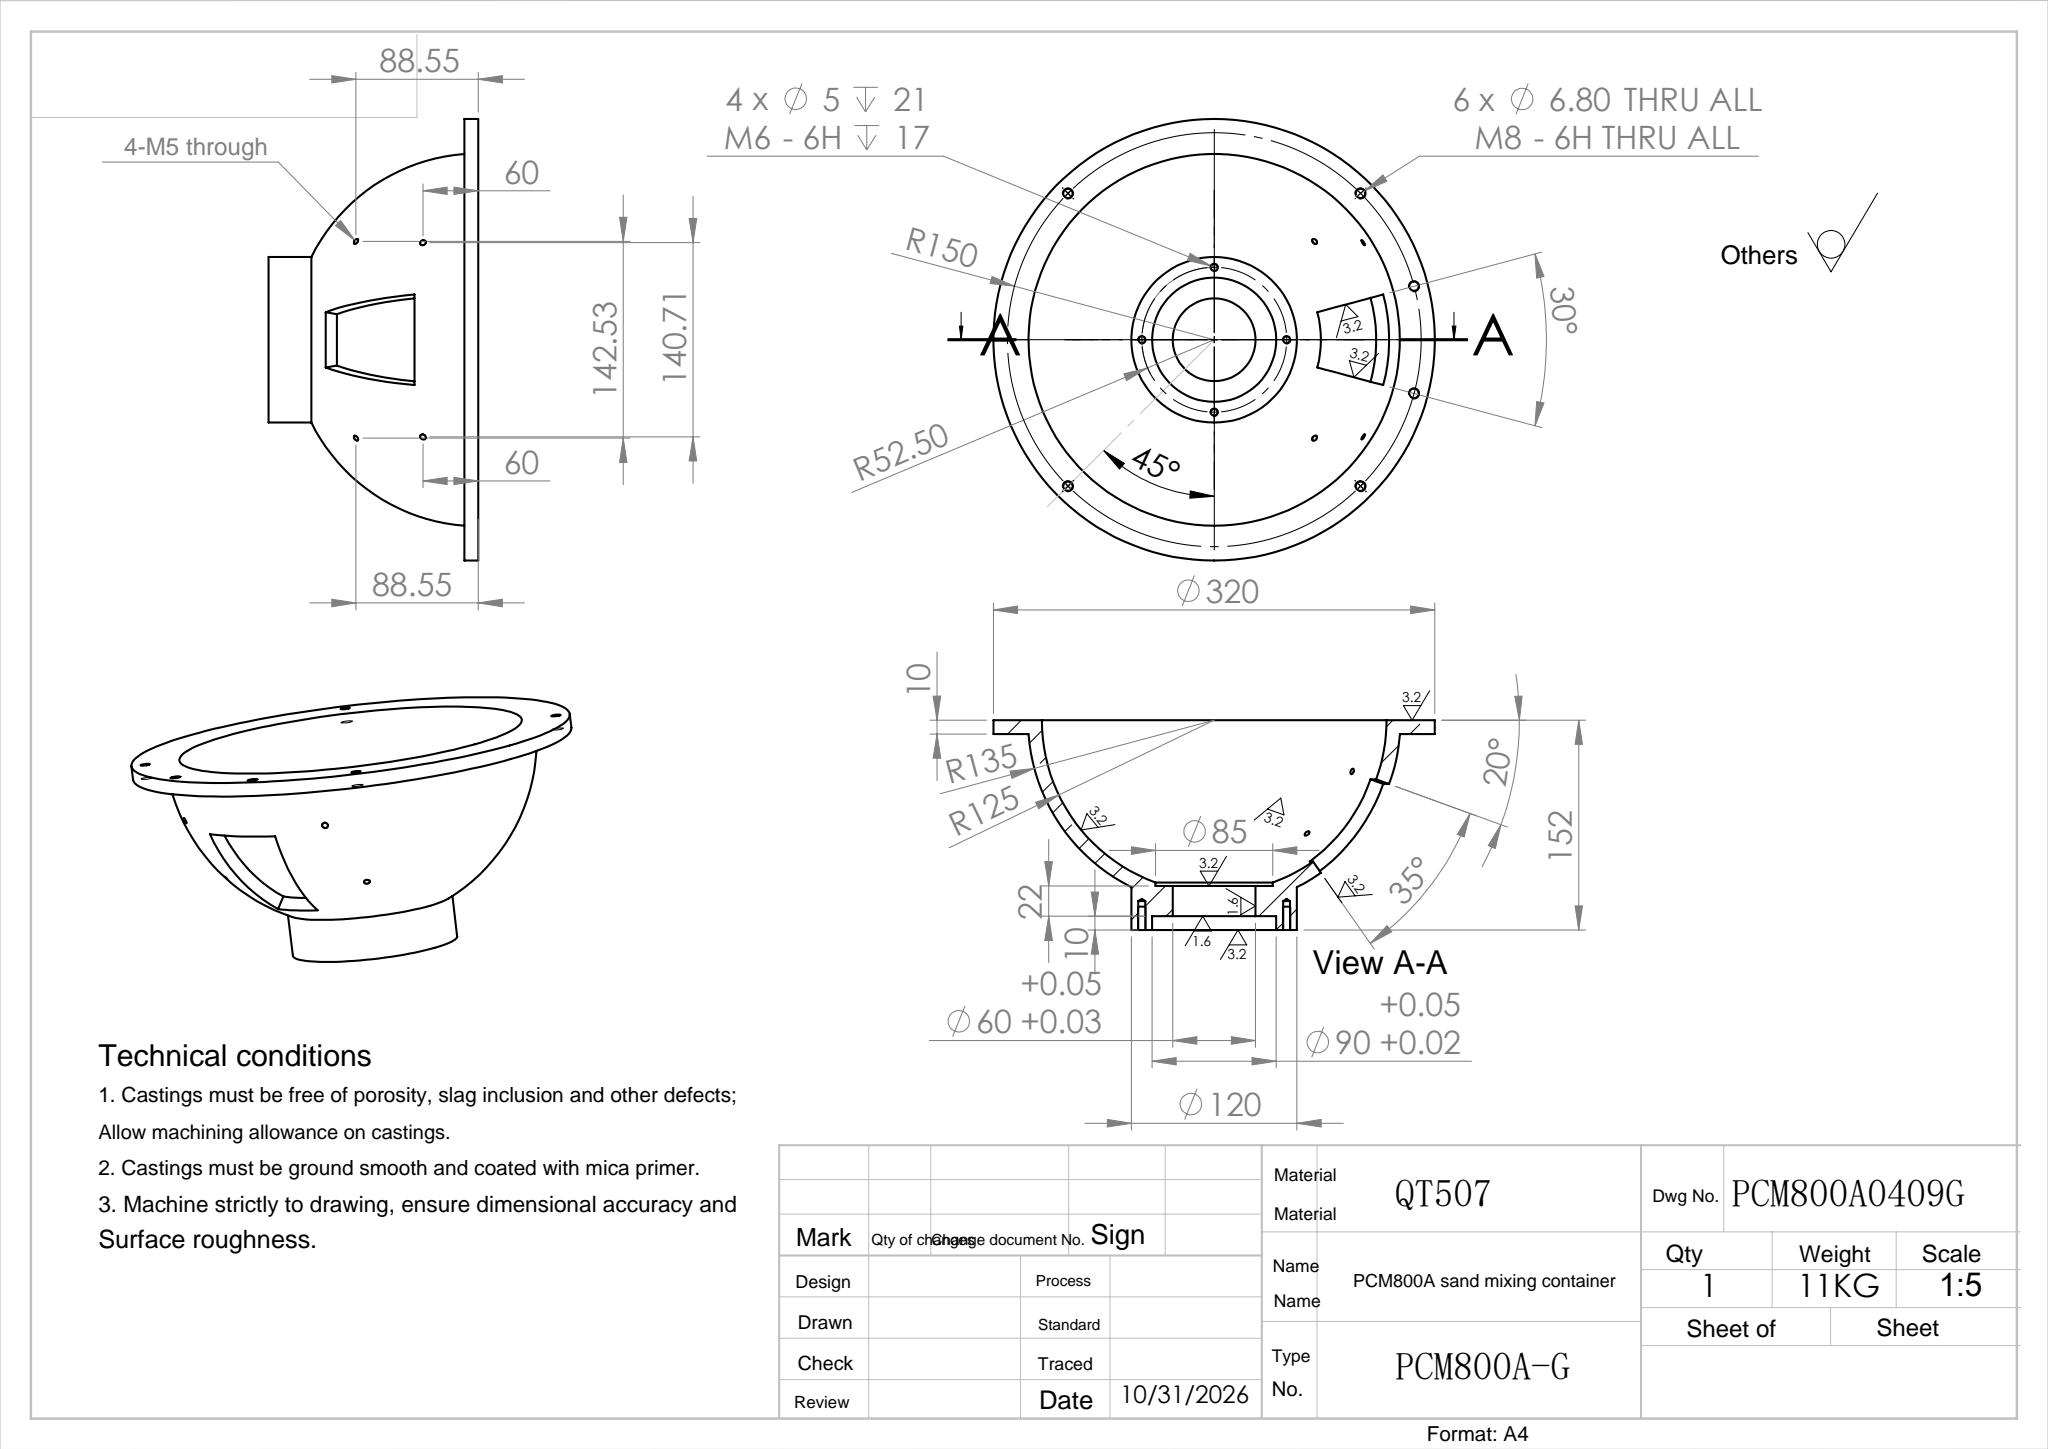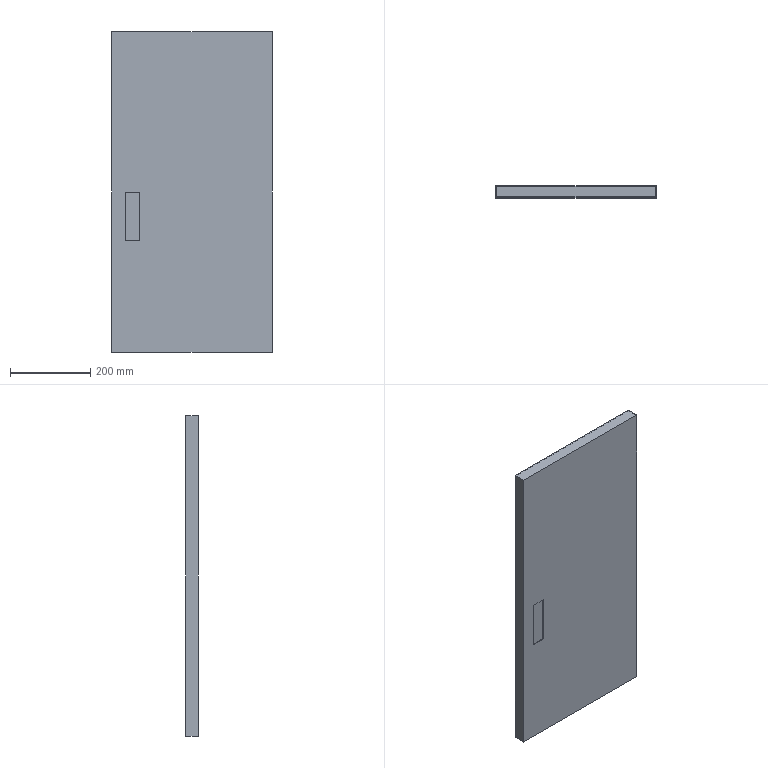Part | SolidWorks | features ICE 2, Extrusion 1, Shell 1 | 1 solid | 16 faces | box 400 x 30 x 800 mm | volume 1395984 mm3 | plane 16
STEP:
#1=CARTESIAN_POINT('',(2.,28.,-798.));
#2=VERTEX_POINT('',#1);
#3=CARTESIAN_POINT('',(2.,2.,-798.));
#4=VERTEX_POINT('',#3);
#5=CARTESIAN_POINT('',(2.,30.,-798.));
#6=DIRECTION('',(0.,-1.,0.));
#7=VECTOR('',#6,1000.);
#8=LINE('',#5,#7);
#9=EDGE_CURVE('',#2,#4,#8,.T.);
#10=ORIENTED_EDGE('',*,*,#9,.F.);
#11=CARTESIAN_POINT('',(2.,28.,-2.));
#12=VERTEX_POINT('',#11);
#13=CARTESIAN_POINT('',(2.,28.,0.));
#14=DIRECTION('',(0.,0.,1.));
#15=VECTOR('',#14,1000.);
#16=LINE('',#13,#15);
#17=EDGE_CURVE('',#2,#12,#16,.T.);
#18=ORIENTED_EDGE('',*,*,#17,.T.);
#19=CARTESIAN_POINT('',(2.,2.,-2.));
#20=VERTEX_POINT('',#19);
#21=CARTESIAN_POINT('',(2.,30.,-2.));
#22=DIRECTION('',(0.,-1.,0.));
#23=VECTOR('',#22,1000.);
#24=LINE('',#21,#23);
#25=EDGE_CURVE('',#12,#20,#24,.T.);
#26=ORIENTED_EDGE('',*,*,#25,.T.);
#27=CARTESIAN_POINT('',(2.,2.,-800.));
#28=DIRECTION('',(0.,0.,1.));
#29=VECTOR('',#28,1000.);
#30=LINE('',#27,#29);
#31=EDGE_CURVE('',#4,#20,#30,.T.);
#32=ORIENTED_EDGE('',*,*,#31,.F.);
#33=EDGE_LOOP('',(#10,#18,#26,#32));
#34=FACE_OUTER_BOUND('',#33,.T.);
#35=CARTESIAN_POINT('',(2.,30.,0.));
#36=DIRECTION('',(1.,0.,0.));
#37=DIRECTION('',(0.,0.,-1.));
#38=AXIS2_PLACEMENT_3D('',#35,#36,#37);
#39=PLANE('',#38);
#40=ADVANCED_FACE('',(#34),#39,.T.);
#41=ORIENTED_EDGE('',*,*,#25,.F.);
#42=CARTESIAN_POINT('',(398.,28.,-2.));
#43=VERTEX_POINT('',#42);
#44=CARTESIAN_POINT('',(0.,28.,-2.));
#45=DIRECTION('',(1.,0.,0.));
#46=VECTOR('',#45,1000.);
#47=LINE('',#44,#46);
#48=EDGE_CURVE('',#12,#43,#47,.T.);
#49=ORIENTED_EDGE('',*,*,#48,.T.);
#50=CARTESIAN_POINT('',(398.,2.,-2.));
#51=VERTEX_POINT('',#50);
#52=CARTESIAN_POINT('',(398.,30.,-2.));
#53=DIRECTION('',(0.,-1.,0.));
#54=VECTOR('',#53,1000.);
#55=LINE('',#52,#54);
#56=EDGE_CURVE('',#43,#51,#55,.T.);
#57=ORIENTED_EDGE('',*,*,#56,.T.);
#58=CARTESIAN_POINT('',(0.,2.,-2.));
#59=DIRECTION('',(1.,0.,0.));
#60=VECTOR('',#59,1000.);
#61=LINE('',#58,#60);
#62=EDGE_CURVE('',#20,#51,#61,.T.);
#63=ORIENTED_EDGE('',*,*,#62,.F.);
#64=EDGE_LOOP('',(#41,#49,#57,#63));
#65=FACE_OUTER_BOUND('',#64,.T.);
#66=CARTESIAN_POINT('',(0.,30.,-2.));
#67=DIRECTION('',(0.,0.,-1.));
#68=DIRECTION('',(-1.,0.,0.));
#69=AXIS2_PLACEMENT_3D('',#66,#67,#68);
#70=PLANE('',#69);
#71=ADVANCED_FACE('',(#65),#70,.T.);
#72=ORIENTED_EDGE('',*,*,#56,.F.);
#73=CARTESIAN_POINT('',(398.,28.,-798.));
#74=VERTEX_POINT('',#73);
#75=CARTESIAN_POINT('',(398.,28.,0.));
#76=DIRECTION('',(0.,0.,-1.));
#77=VECTOR('',#76,1000.);
#78=LINE('',#75,#77);
#79=EDGE_CURVE('',#43,#74,#78,.T.);
#80=ORIENTED_EDGE('',*,*,#79,.T.);
#81=CARTESIAN_POINT('',(398.,2.,-798.));
#82=VERTEX_POINT('',#81);
#83=CARTESIAN_POINT('',(398.,30.,-798.));
#84=DIRECTION('',(0.,-1.,0.));
#85=VECTOR('',#84,1000.);
#86=LINE('',#83,#85);
#87=EDGE_CURVE('',#74,#82,#86,.T.);
#88=ORIENTED_EDGE('',*,*,#87,.T.);
#89=CARTESIAN_POINT('',(398.,2.,-800.));
#90=DIRECTION('',(0.,0.,-1.));
#91=VECTOR('',#90,1000.);
#92=LINE('',#89,#91);
#93=EDGE_CURVE('',#51,#82,#92,.T.);
#94=ORIENTED_EDGE('',*,*,#93,.F.);
#95=EDGE_LOOP('',(#72,#80,#88,#94));
#96=FACE_OUTER_BOUND('',#95,.T.);
#97=CARTESIAN_POINT('',(398.,30.,0.));
#98=DIRECTION('',(-1.,0.,0.));
#99=DIRECTION('',(0.,0.,1.));
#100=AXIS2_PLACEMENT_3D('',#97,#98,#99);
#101=PLANE('',#100);
#102=ADVANCED_FACE('',(#96),#101,.T.);
#103=ORIENTED_EDGE('',*,*,#87,.F.);
#104=CARTESIAN_POINT('',(0.,28.,-798.));
#105=DIRECTION('',(-1.,0.,0.));
#106=VECTOR('',#105,1000.);
#107=LINE('',#104,#106);
#108=EDGE_CURVE('',#74,#2,#107,.T.);
#109=ORIENTED_EDGE('',*,*,#108,.T.);
#110=ORIENTED_EDGE('',*,*,#9,.T.);
#111=CARTESIAN_POINT('',(0.,2.,-798.));
#112=DIRECTION('',(-1.,0.,0.));
#113=VECTOR('',#112,1000.);
#114=LINE('',#111,#113);
#115=EDGE_CURVE('',#82,#4,#114,.T.);
#116=ORIENTED_EDGE('',*,*,#115,.F.);
#117=EDGE_LOOP('',(#103,#109,#110,#116));
#118=FACE_OUTER_BOUND('',#117,.T.);
#119=CARTESIAN_POINT('',(0.,30.,-798.));
#120=DIRECTION('',(0.,0.,1.));
#121=DIRECTION('',(1.,0.,0.));
#122=AXIS2_PLACEMENT_3D('',#119,#120,#121);
#123=PLANE('',#122);
#124=ADVANCED_FACE('',(#118),#123,.T.);
#125=CARTESIAN_POINT('',(0.,30.,-800.));
#126=VERTEX_POINT('',#125);
#127=CARTESIAN_POINT('',(0.,30.,0.));
#128=VERTEX_POINT('',#127);
#129=CARTESIAN_POINT('',(0.,30.,0.));
#130=DIRECTION('',(0.,0.,1.));
#131=VECTOR('',#130,1000.);
#132=LINE('',#129,#131);
#133=EDGE_CURVE('',#126,#128,#132,.T.);
#134=ORIENTED_EDGE('',*,*,#133,.T.);
#135=CARTESIAN_POINT('',(400.,30.,0.));
#136=VERTEX_POINT('',#135);
#137=CARTESIAN_POINT('',(0.,30.,0.));
#138=DIRECTION('',(1.,0.,0.));
#139=VECTOR('',#138,1000.);
#140=LINE('',#137,#139);
#141=EDGE_CURVE('',#128,#136,#140,.T.);
#142=ORIENTED_EDGE('',*,*,#141,.T.);
#143=CARTESIAN_POINT('',(400.,30.,-800.));
#144=VERTEX_POINT('',#143);
#145=CARTESIAN_POINT('',(400.,30.,0.));
#146=DIRECTION('',(0.,0.,-1.));
#147=VECTOR('',#146,1000.);
#148=LINE('',#145,#147);
#149=EDGE_CURVE('',#136,#144,#148,.T.);
#150=ORIENTED_EDGE('',*,*,#149,.T.);
#151=CARTESIAN_POINT('',(0.,30.,-800.));
#152=DIRECTION('',(-1.,0.,0.));
#153=VECTOR('',#152,1000.);
#154=LINE('',#151,#153);
#155=EDGE_CURVE('',#144,#126,#154,.T.);
#156=ORIENTED_EDGE('',*,*,#155,.T.);
#157=EDGE_LOOP('',(#134,#142,#150,#156));
#158=FACE_OUTER_BOUND('',#157,.T.);
#159=CARTESIAN_POINT('',(0.,30.,-800.));
#160=DIRECTION('',(0.,-1.,0.));
#161=DIRECTION('',(0.,0.,-1.));
#162=AXIS2_PLACEMENT_3D('',#159,#160,#161);
#163=PLANE('',#162);
#164=ADVANCED_FACE('',(#158),#163,.F.);
#165=CARTESIAN_POINT('',(0.,0.,-800.));
#166=VERTEX_POINT('',#165);
#167=CARTESIAN_POINT('',(0.,30.,-800.));
#168=DIRECTION('',(0.,-1.,0.));
#169=VECTOR('',#168,1000.);
#170=LINE('',#167,#169);
#171=EDGE_CURVE('',#126,#166,#170,.T.);
#172=ORIENTED_EDGE('',*,*,#171,.T.);
#173=CARTESIAN_POINT('',(0.,0.,0.));
#174=VERTEX_POINT('',#173);
#175=CARTESIAN_POINT('',(0.,0.,0.));
#176=DIRECTION('',(0.,0.,1.));
#177=VECTOR('',#176,1000.);
#178=LINE('',#175,#177);
#179=EDGE_CURVE('',#166,#174,#178,.T.);
#180=ORIENTED_EDGE('',*,*,#179,.T.);
#181=CARTESIAN_POINT('',(0.,30.,0.));
#182=DIRECTION('',(0.,-1.,0.));
#183=VECTOR('',#182,1000.);
#184=LINE('',#181,#183);
#185=EDGE_CURVE('',#128,#174,#184,.T.);
#186=ORIENTED_EDGE('',*,*,#185,.F.);
#187=ORIENTED_EDGE('',*,*,#133,.F.);
#188=EDGE_LOOP('',(#172,#180,#186,#187));
#189=FACE_OUTER_BOUND('',#188,.T.);
#190=CARTESIAN_POINT('',(0.,30.,0.));
#191=DIRECTION('',(1.,0.,0.));
#192=DIRECTION('',(0.,0.,-1.));
#193=AXIS2_PLACEMENT_3D('',#190,#191,#192);
#194=PLANE('',#193);
#195=ADVANCED_FACE('',(#189),#194,.F.);
#196=ORIENTED_EDGE('',*,*,#185,.T.);
#197=CARTESIAN_POINT('',(400.,0.,0.));
#198=VERTEX_POINT('',#197);
#199=CARTESIAN_POINT('',(0.,0.,0.));
#200=DIRECTION('',(1.,0.,0.));
#201=VECTOR('',#200,1000.);
#202=LINE('',#199,#201);
#203=EDGE_CURVE('',#174,#198,#202,.T.);
#204=ORIENTED_EDGE('',*,*,#203,.T.);
#205=CARTESIAN_POINT('',(400.,30.,0.));
#206=DIRECTION('',(0.,-1.,0.));
#207=VECTOR('',#206,1000.);
#208=LINE('',#205,#207);
#209=EDGE_CURVE('',#136,#198,#208,.T.);
#210=ORIENTED_EDGE('',*,*,#209,.F.);
#211=ORIENTED_EDGE('',*,*,#141,.F.);
#212=EDGE_LOOP('',(#196,#204,#210,#211));
#213=FACE_OUTER_BOUND('',#212,.T.);
#214=CARTESIAN_POINT('',(0.,30.,0.));
#215=DIRECTION('',(0.,0.,-1.));
#216=DIRECTION('',(-1.,0.,0.));
#217=AXIS2_PLACEMENT_3D('',#214,#215,#216);
#218=PLANE('',#217);
#219=ADVANCED_FACE('',(#213),#218,.F.);
#220=ORIENTED_EDGE('',*,*,#209,.T.);
#221=CARTESIAN_POINT('',(400.,0.,-800.));
#222=VERTEX_POINT('',#221);
#223=CARTESIAN_POINT('',(400.,0.,0.));
#224=DIRECTION('',(0.,0.,-1.));
#225=VECTOR('',#224,1000.);
#226=LINE('',#223,#225);
#227=EDGE_CURVE('',#198,#222,#226,.T.);
#228=ORIENTED_EDGE('',*,*,#227,.T.);
#229=CARTESIAN_POINT('',(400.,30.,-800.));
#230=DIRECTION('',(0.,-1.,0.));
#231=VECTOR('',#230,1000.);
#232=LINE('',#229,#231);
#233=EDGE_CURVE('',#144,#222,#232,.T.);
#234=ORIENTED_EDGE('',*,*,#233,.F.);
#235=ORIENTED_EDGE('',*,*,#149,.F.);
#236=EDGE_LOOP('',(#220,#228,#234,#235));
#237=FACE_OUTER_BOUND('',#236,.T.);
#238=CARTESIAN_POINT('',(400.,30.,0.));
#239=DIRECTION('',(-1.,0.,0.));
#240=DIRECTION('',(0.,0.,1.));
#241=AXIS2_PLACEMENT_3D('',#238,#239,#240);
#242=PLANE('',#241);
#243=ADVANCED_FACE('',(#237),#242,.F.);
#244=ORIENTED_EDGE('',*,*,#233,.T.);
#245=CARTESIAN_POINT('',(0.,0.,-800.));
#246=DIRECTION('',(-1.,0.,0.));
#247=VECTOR('',#246,1000.);
#248=LINE('',#245,#247);
#249=EDGE_CURVE('',#222,#166,#248,.T.);
#250=ORIENTED_EDGE('',*,*,#249,.T.);
#251=ORIENTED_EDGE('',*,*,#171,.F.);
#252=ORIENTED_EDGE('',*,*,#155,.F.);
#253=EDGE_LOOP('',(#244,#250,#251,#252));
#254=FACE_OUTER_BOUND('',#253,.T.);
#255=CARTESIAN_POINT('',(0.,30.,-800.));
#256=DIRECTION('',(0.,0.,1.));
#257=DIRECTION('',(1.,0.,0.));
#258=AXIS2_PLACEMENT_3D('',#255,#256,#257);
#259=PLANE('',#258);
#260=ADVANCED_FACE('',(#254),#259,.F.);
#261=CARTESIAN_POINT('',(70.,0.,-520.));
#262=VERTEX_POINT('',#261);
#263=CARTESIAN_POINT('',(70.,0.,-400.));
#264=VERTEX_POINT('',#263);
#265=CARTESIAN_POINT('',(70.,0.,-520.));
#266=DIRECTION('',(0.,0.,1.));
#267=VECTOR('',#266,1000.);
#268=LINE('',#265,#267);
#269=EDGE_CURVE('',#262,#264,#268,.T.);
#270=ORIENTED_EDGE('',*,*,#269,.F.);
#271=CARTESIAN_POINT('',(35.,0.,-520.));
#272=VERTEX_POINT('',#271);
#273=CARTESIAN_POINT('',(70.,0.,-520.));
#274=DIRECTION('',(1.,0.,0.));
#275=VECTOR('',#274,1000.);
#276=LINE('',#273,#275);
#277=EDGE_CURVE('',#272,#262,#276,.T.);
#278=ORIENTED_EDGE('',*,*,#277,.F.);
#279=CARTESIAN_POINT('',(35.,0.,-400.));
#280=VERTEX_POINT('',#279);
#281=CARTESIAN_POINT('',(35.,0.,-520.));
#282=DIRECTION('',(0.,0.,-1.));
#283=VECTOR('',#282,1000.);
#284=LINE('',#281,#283);
#285=EDGE_CURVE('',#280,#272,#284,.T.);
#286=ORIENTED_EDGE('',*,*,#285,.F.);
#287=CARTESIAN_POINT('',(70.,0.,-400.));
#288=DIRECTION('',(-1.,0.,0.));
#289=VECTOR('',#288,1000.);
#290=LINE('',#287,#289);
#291=EDGE_CURVE('',#264,#280,#290,.T.);
#292=ORIENTED_EDGE('',*,*,#291,.F.);
#293=EDGE_LOOP('',(#270,#278,#286,#292));
#294=FACE_BOUND('',#293,.T.);
#295=ORIENTED_EDGE('',*,*,#179,.F.);
#296=ORIENTED_EDGE('',*,*,#249,.F.);
#297=ORIENTED_EDGE('',*,*,#227,.F.);
#298=ORIENTED_EDGE('',*,*,#203,.F.);
#299=EDGE_LOOP('',(#295,#296,#297,#298));
#300=FACE_OUTER_BOUND('',#299,.T.);
#301=CARTESIAN_POINT('',(0.,0.,-800.));
#302=DIRECTION('',(0.,-1.,0.));
#303=DIRECTION('',(0.,0.,-1.));
#304=AXIS2_PLACEMENT_3D('',#301,#302,#303);
#305=PLANE('',#304);
#306=ADVANCED_FACE('',(#294,#300),#305,.T.);
#307=CARTESIAN_POINT('',(35.,2.,-520.));
#308=VERTEX_POINT('',#307);
#309=CARTESIAN_POINT('',(70.,2.,-520.));
#310=VERTEX_POINT('',#309);
#311=CARTESIAN_POINT('',(0.,2.,-520.));
#312=DIRECTION('',(1.,0.,0.));
#313=VECTOR('',#312,1000.);
#314=LINE('',#311,#313);
#315=EDGE_CURVE('',#308,#310,#314,.T.);
#316=ORIENTED_EDGE('',*,*,#315,.T.);
#317=CARTESIAN_POINT('',(70.,2.,-400.));
#318=VERTEX_POINT('',#317);
#319=CARTESIAN_POINT('',(70.,2.,-800.));
#320=DIRECTION('',(0.,0.,1.));
#321=VECTOR('',#320,1000.);
#322=LINE('',#319,#321);
#323=EDGE_CURVE('',#310,#318,#322,.T.);
#324=ORIENTED_EDGE('',*,*,#323,.T.);
#325=CARTESIAN_POINT('',(35.,2.,-400.));
#326=VERTEX_POINT('',#325);
#327=CARTESIAN_POINT('',(0.,2.,-400.));
#328=DIRECTION('',(-1.,0.,0.));
#329=VECTOR('',#328,1000.);
#330=LINE('',#327,#329);
#331=EDGE_CURVE('',#318,#326,#330,.T.);
#332=ORIENTED_EDGE('',*,*,#331,.T.);
#333=CARTESIAN_POINT('',(35.,2.,-800.));
#334=DIRECTION('',(0.,0.,-1.));
#335=VECTOR('',#334,1000.);
#336=LINE('',#333,#335);
#337=EDGE_CURVE('',#326,#308,#336,.T.);
#338=ORIENTED_EDGE('',*,*,#337,.T.);
#339=EDGE_LOOP('',(#316,#324,#332,#338));
#340=FACE_BOUND('',#339,.T.);
#341=ORIENTED_EDGE('',*,*,#31,.T.);
#342=ORIENTED_EDGE('',*,*,#62,.T.);
#343=ORIENTED_EDGE('',*,*,#93,.T.);
#344=ORIENTED_EDGE('',*,*,#115,.T.);
#345=EDGE_LOOP('',(#341,#342,#343,#344));
#346=FACE_OUTER_BOUND('',#345,.T.);
#347=CARTESIAN_POINT('',(0.,2.,-800.));
#348=DIRECTION('',(0.,-1.,0.));
#349=DIRECTION('',(0.,0.,-1.));
#350=AXIS2_PLACEMENT_3D('',#347,#348,#349);
#351=PLANE('',#350);
#352=ADVANCED_FACE('',(#340,#346),#351,.F.);
#353=CARTESIAN_POINT('',(70.,28.,-520.));
#354=DIRECTION('',(0.,-1.,0.));
#355=VECTOR('',#354,1000.);
#356=LINE('',#353,#355);
#357=EDGE_CURVE('',#310,#262,#356,.T.);
#358=ORIENTED_EDGE('',*,*,#357,.T.);
#359=ORIENTED_EDGE('',*,*,#269,.T.);
#360=CARTESIAN_POINT('',(70.,28.,-400.));
#361=DIRECTION('',(0.,-1.,0.));
#362=VECTOR('',#361,1000.);
#363=LINE('',#360,#362);
#364=EDGE_CURVE('',#318,#264,#363,.T.);
#365=ORIENTED_EDGE('',*,*,#364,.F.);
#366=ORIENTED_EDGE('',*,*,#323,.F.);
#367=EDGE_LOOP('',(#358,#359,#365,#366));
#368=FACE_OUTER_BOUND('',#367,.T.);
#369=CARTESIAN_POINT('',(70.,28.,-520.));
#370=DIRECTION('',(1.,0.,0.));
#371=DIRECTION('',(0.,0.,-1.));
#372=AXIS2_PLACEMENT_3D('',#369,#370,#371);
#373=PLANE('',#372);
#374=ADVANCED_FACE('',(#368),#373,.F.);
#375=CARTESIAN_POINT('',(35.,28.,-520.));
#376=DIRECTION('',(0.,-1.,0.));
#377=VECTOR('',#376,1000.);
#378=LINE('',#375,#377);
#379=EDGE_CURVE('',#308,#272,#378,.T.);
#380=ORIENTED_EDGE('',*,*,#379,.T.);
#381=ORIENTED_EDGE('',*,*,#277,.T.);
#382=ORIENTED_EDGE('',*,*,#357,.F.);
#383=ORIENTED_EDGE('',*,*,#315,.F.);
#384=EDGE_LOOP('',(#380,#381,#382,#383));
#385=FACE_OUTER_BOUND('',#384,.T.);
#386=CARTESIAN_POINT('',(70.,28.,-520.));
#387=DIRECTION('',(0.,0.,-1.));
#388=DIRECTION('',(-1.,0.,0.));
#389=AXIS2_PLACEMENT_3D('',#386,#387,#388);
#390=PLANE('',#389);
#391=ADVANCED_FACE('',(#385),#390,.F.);
#392=CARTESIAN_POINT('',(35.,28.,-400.));
#393=DIRECTION('',(0.,-1.,0.));
#394=VECTOR('',#393,1000.);
#395=LINE('',#392,#394);
#396=EDGE_CURVE('',#326,#280,#395,.T.);
#397=ORIENTED_EDGE('',*,*,#396,.T.);
#398=ORIENTED_EDGE('',*,*,#285,.T.);
#399=ORIENTED_EDGE('',*,*,#379,.F.);
#400=ORIENTED_EDGE('',*,*,#337,.F.);
#401=EDGE_LOOP('',(#397,#398,#399,#400));
#402=FACE_OUTER_BOUND('',#401,.T.);
#403=CARTESIAN_POINT('',(35.,28.,-520.));
#404=DIRECTION('',(-1.,0.,0.));
#405=DIRECTION('',(0.,0.,1.));
#406=AXIS2_PLACEMENT_3D('',#403,#404,#405);
#407=PLANE('',#406);
#408=ADVANCED_FACE('',(#402),#407,.F.);
#409=ORIENTED_EDGE('',*,*,#364,.T.);
#410=ORIENTED_EDGE('',*,*,#291,.T.);
#411=ORIENTED_EDGE('',*,*,#396,.F.);
#412=ORIENTED_EDGE('',*,*,#331,.F.);
#413=EDGE_LOOP('',(#409,#410,#411,#412));
#414=FACE_OUTER_BOUND('',#413,.T.);
#415=CARTESIAN_POINT('',(70.,28.,-400.));
#416=DIRECTION('',(0.,0.,1.));
#417=DIRECTION('',(1.,0.,0.));
#418=AXIS2_PLACEMENT_3D('',#415,#416,#417);
#419=PLANE('',#418);
#420=ADVANCED_FACE('',(#414),#419,.F.);
#421=ORIENTED_EDGE('',*,*,#17,.F.);
#422=ORIENTED_EDGE('',*,*,#108,.F.);
#423=ORIENTED_EDGE('',*,*,#79,.F.);
#424=ORIENTED_EDGE('',*,*,#48,.F.);
#425=EDGE_LOOP('',(#421,#422,#423,#424));
#426=FACE_OUTER_BOUND('',#425,.T.);
#427=CARTESIAN_POINT('',(0.,28.,0.));
#428=DIRECTION('',(0.,1.,0.));
#429=DIRECTION('',(0.,0.,1.));
#430=AXIS2_PLACEMENT_3D('',#427,#428,#429);
#431=PLANE('',#430);
#432=ADVANCED_FACE('',(#426),#431,.F.);
#433=CLOSED_SHELL('',(#40,#71,#102,#124,#164,#195,#219,#243,#260,#306,#352,#374,#391,#408,#420,#432));
#434=MANIFOLD_SOLID_BREP('',#433);
#435=CARTESIAN_POINT('',(0.,0.,0.));
#436=DIRECTION('',(0.,0.,1.));
#437=DIRECTION('',(1.,0.,0.));
#438=AXIS2_PLACEMENT_3D('',#435,#436,#437);
#439=(LENGTH_UNIT()NAMED_UNIT(*)SI_UNIT(.MILLI.,.METRE.));
#440=UNCERTAINTY_MEASURE_WITH_UNIT(LENGTH_MEASURE(0.00001),#439,'','');
#441=(NAMED_UNIT(*)PLANE_ANGLE_UNIT()SI_UNIT($,.RADIAN.));
#442=(NAMED_UNIT(*)SI_UNIT($,.STERADIAN.)SOLID_ANGLE_UNIT());
#443=(GEOMETRIC_REPRESENTATION_CONTEXT(3)GLOBAL_UNCERTAINTY_ASSIGNED_CONTEXT((#440))GLOBAL_UNIT_ASSIGNED_CONTEXT((#439,#441,#442))REPRESENTATION_CONTEXT('',''));
#444=ADVANCED_BREP_SHAPE_REPRESENTATION('',(#434,#438),#443);